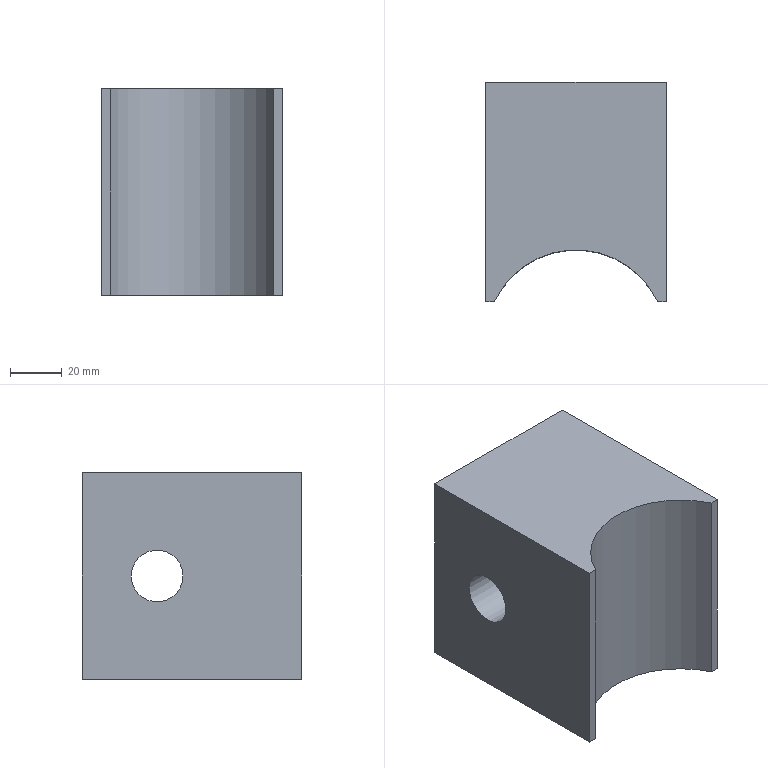Part | NX | features 护邦千斤顶滑块 2 | 1 solid | 9 faces | box 70 x 85 x 80 mm | volume 381423 mm3 | plane 7 | cylinder 2 | commonest cylinder face diameters 20 x1 70 x1
STEP:
#1=CARTESIAN_POINT('',(0.,-39.,40.));
#2=VERTEX_POINT('',#1);
#3=CARTESIAN_POINT('',(0.,-29.,40.));
#4=DIRECTION('',(-1.,0.,0.));
#5=DIRECTION('',(0.,-1.,0.));
#6=AXIS2_PLACEMENT_3D('',#3,#4,#5);
#7=CIRCLE('',#6,10.);
#8=EDGE_CURVE('',#2,#2,#7,.T.);
#9=ORIENTED_EDGE('',*,*,#8,.F.);
#10=EDGE_LOOP('',(#9));
#11=FACE_BOUND('',#10,.T.);
#12=CARTESIAN_POINT('',(0.,0.,0.));
#13=VERTEX_POINT('',#12);
#14=CARTESIAN_POINT('',(0.,-85.,0.));
#15=VERTEX_POINT('',#14);
#16=CARTESIAN_POINT('',(0.,0.,0.));
#17=DIRECTION('',(0.,-1.,0.));
#18=VECTOR('',#17,1000.);
#19=LINE('',#16,#18);
#20=EDGE_CURVE('',#13,#15,#19,.T.);
#21=ORIENTED_EDGE('',*,*,#20,.T.);
#22=CARTESIAN_POINT('',(0.,-85.,80.));
#23=VERTEX_POINT('',#22);
#24=CARTESIAN_POINT('',(0.,-85.,80.));
#25=DIRECTION('',(0.,0.,-1.));
#26=VECTOR('',#25,1000.);
#27=LINE('',#24,#26);
#28=EDGE_CURVE('',#23,#15,#27,.T.);
#29=ORIENTED_EDGE('',*,*,#28,.F.);
#30=CARTESIAN_POINT('',(0.,0.,80.));
#31=VERTEX_POINT('',#30);
#32=CARTESIAN_POINT('',(0.,0.,80.));
#33=DIRECTION('',(0.,-1.,0.));
#34=VECTOR('',#33,1000.);
#35=LINE('',#32,#34);
#36=EDGE_CURVE('',#31,#23,#35,.T.);
#37=ORIENTED_EDGE('',*,*,#36,.F.);
#38=CARTESIAN_POINT('',(0.,0.,80.));
#39=DIRECTION('',(0.,0.,-1.));
#40=VECTOR('',#39,1000.);
#41=LINE('',#38,#40);
#42=EDGE_CURVE('',#31,#13,#41,.T.);
#43=ORIENTED_EDGE('',*,*,#42,.T.);
#44=EDGE_LOOP('',(#21,#29,#37,#43));
#45=FACE_BOUND('',#44,.T.);
#46=CARTESIAN_POINT('',(0.,0.,80.));
#47=DIRECTION('',(1.,0.,0.));
#48=DIRECTION('',(0.,1.,0.));
#49=AXIS2_PLACEMENT_3D('',#46,#47,#48);
#50=PLANE('',#49);
#51=ADVANCED_FACE('',(#11,#45),#50,.F.);
#52=CARTESIAN_POINT('',(3.377,-85.,0.));
#53=VERTEX_POINT('',#52);
#54=CARTESIAN_POINT('',(0.,-85.,0.));
#55=DIRECTION('',(1.,0.,0.));
#56=VECTOR('',#55,1000.);
#57=LINE('',#54,#56);
#58=EDGE_CURVE('',#15,#53,#57,.T.);
#59=ORIENTED_EDGE('',*,*,#58,.T.);
#60=CARTESIAN_POINT('',(3.377,-85.,80.));
#61=VERTEX_POINT('',#60);
#62=CARTESIAN_POINT('',(3.377,-85.,80.));
#63=DIRECTION('',(0.,0.,-1.));
#64=VECTOR('',#63,1000.);
#65=LINE('',#62,#64);
#66=EDGE_CURVE('',#61,#53,#65,.T.);
#67=ORIENTED_EDGE('',*,*,#66,.F.);
#68=CARTESIAN_POINT('',(0.,-85.,80.));
#69=DIRECTION('',(1.,0.,0.));
#70=VECTOR('',#69,1000.);
#71=LINE('',#68,#70);
#72=EDGE_CURVE('',#23,#61,#71,.T.);
#73=ORIENTED_EDGE('',*,*,#72,.F.);
#74=ORIENTED_EDGE('',*,*,#28,.T.);
#75=EDGE_LOOP('',(#59,#67,#73,#74));
#76=FACE_BOUND('',#75,.T.);
#77=CARTESIAN_POINT('',(0.,-85.,80.));
#78=DIRECTION('',(0.,1.,0.));
#79=DIRECTION('',(0.,0.,1.));
#80=AXIS2_PLACEMENT_3D('',#77,#78,#79);
#81=PLANE('',#80);
#82=ADVANCED_FACE('',(#76),#81,.F.);
#83=CARTESIAN_POINT('',(66.623,-85.,0.));
#84=VERTEX_POINT('',#83);
#85=CARTESIAN_POINT('',(35.,-100.,0.));
#86=DIRECTION('',(0.,0.,-1.));
#87=DIRECTION('',(1.,0.,0.));
#88=AXIS2_PLACEMENT_3D('',#85,#86,#87);
#89=CIRCLE('',#88,35.);
#90=EDGE_CURVE('',#53,#84,#89,.T.);
#91=ORIENTED_EDGE('',*,*,#90,.T.);
#92=CARTESIAN_POINT('',(66.623,-85.,80.));
#93=VERTEX_POINT('',#92);
#94=CARTESIAN_POINT('',(66.623,-85.,80.));
#95=DIRECTION('',(0.,0.,-1.));
#96=VECTOR('',#95,1000.);
#97=LINE('',#94,#96);
#98=EDGE_CURVE('',#93,#84,#97,.T.);
#99=ORIENTED_EDGE('',*,*,#98,.F.);
#100=CARTESIAN_POINT('',(35.,-100.,80.));
#101=DIRECTION('',(0.,0.,-1.));
#102=DIRECTION('',(1.,0.,0.));
#103=AXIS2_PLACEMENT_3D('',#100,#101,#102);
#104=CIRCLE('',#103,35.);
#105=EDGE_CURVE('',#61,#93,#104,.T.);
#106=ORIENTED_EDGE('',*,*,#105,.F.);
#107=ORIENTED_EDGE('',*,*,#66,.T.);
#108=EDGE_LOOP('',(#91,#99,#106,#107));
#109=FACE_BOUND('',#108,.T.);
#110=CARTESIAN_POINT('',(35.,-100.,80.));
#111=DIRECTION('',(0.,0.,-1.));
#112=DIRECTION('',(-1.,0.,0.));
#113=AXIS2_PLACEMENT_3D('',#110,#111,#112);
#114=CYLINDRICAL_SURFACE('',#113,35.);
#115=ADVANCED_FACE('',(#109),#114,.F.);
#116=CARTESIAN_POINT('',(70.,-85.,0.));
#117=VERTEX_POINT('',#116);
#118=CARTESIAN_POINT('',(66.623,-85.,0.));
#119=DIRECTION('',(1.,0.,0.));
#120=VECTOR('',#119,1000.);
#121=LINE('',#118,#120);
#122=EDGE_CURVE('',#84,#117,#121,.T.);
#123=ORIENTED_EDGE('',*,*,#122,.T.);
#124=CARTESIAN_POINT('',(70.,-85.,80.));
#125=VERTEX_POINT('',#124);
#126=CARTESIAN_POINT('',(70.,-85.,80.));
#127=DIRECTION('',(0.,0.,-1.));
#128=VECTOR('',#127,1000.);
#129=LINE('',#126,#128);
#130=EDGE_CURVE('',#125,#117,#129,.T.);
#131=ORIENTED_EDGE('',*,*,#130,.F.);
#132=CARTESIAN_POINT('',(66.623,-85.,80.));
#133=DIRECTION('',(1.,0.,0.));
#134=VECTOR('',#133,1000.);
#135=LINE('',#132,#134);
#136=EDGE_CURVE('',#93,#125,#135,.T.);
#137=ORIENTED_EDGE('',*,*,#136,.F.);
#138=ORIENTED_EDGE('',*,*,#98,.T.);
#139=EDGE_LOOP('',(#123,#131,#137,#138));
#140=FACE_BOUND('',#139,.T.);
#141=CARTESIAN_POINT('',(66.623,-85.,80.));
#142=DIRECTION('',(0.,1.,0.));
#143=DIRECTION('',(0.,0.,1.));
#144=AXIS2_PLACEMENT_3D('',#141,#142,#143);
#145=PLANE('',#144);
#146=ADVANCED_FACE('',(#140),#145,.F.);
#147=CARTESIAN_POINT('',(70.,-39.,40.));
#148=VERTEX_POINT('',#147);
#149=CARTESIAN_POINT('',(70.,-29.,40.));
#150=DIRECTION('',(-1.,0.,0.));
#151=DIRECTION('',(0.,-1.,0.));
#152=AXIS2_PLACEMENT_3D('',#149,#150,#151);
#153=CIRCLE('',#152,10.);
#154=EDGE_CURVE('',#148,#148,#153,.T.);
#155=ORIENTED_EDGE('',*,*,#154,.T.);
#156=EDGE_LOOP('',(#155));
#157=FACE_BOUND('',#156,.T.);
#158=CARTESIAN_POINT('',(70.,0.,0.));
#159=VERTEX_POINT('',#158);
#160=CARTESIAN_POINT('',(70.,0.,0.));
#161=DIRECTION('',(0.,1.,0.));
#162=VECTOR('',#161,1000.);
#163=LINE('',#160,#162);
#164=EDGE_CURVE('',#117,#159,#163,.T.);
#165=ORIENTED_EDGE('',*,*,#164,.T.);
#166=CARTESIAN_POINT('',(70.,0.,80.));
#167=VERTEX_POINT('',#166);
#168=CARTESIAN_POINT('',(70.,0.,80.));
#169=DIRECTION('',(0.,0.,-1.));
#170=VECTOR('',#169,1000.);
#171=LINE('',#168,#170);
#172=EDGE_CURVE('',#167,#159,#171,.T.);
#173=ORIENTED_EDGE('',*,*,#172,.F.);
#174=CARTESIAN_POINT('',(70.,0.,80.));
#175=DIRECTION('',(0.,1.,0.));
#176=VECTOR('',#175,1000.);
#177=LINE('',#174,#176);
#178=EDGE_CURVE('',#125,#167,#177,.T.);
#179=ORIENTED_EDGE('',*,*,#178,.F.);
#180=ORIENTED_EDGE('',*,*,#130,.T.);
#181=EDGE_LOOP('',(#165,#173,#179,#180));
#182=FACE_BOUND('',#181,.T.);
#183=CARTESIAN_POINT('',(70.,0.,80.));
#184=DIRECTION('',(-1.,0.,0.));
#185=DIRECTION('',(0.,-1.,0.));
#186=AXIS2_PLACEMENT_3D('',#183,#184,#185);
#187=PLANE('',#186);
#188=ADVANCED_FACE('',(#157,#182),#187,.F.);
#189=CARTESIAN_POINT('',(0.,0.,0.));
#190=DIRECTION('',(-1.,0.,0.));
#191=VECTOR('',#190,1000.);
#192=LINE('',#189,#191);
#193=EDGE_CURVE('',#159,#13,#192,.T.);
#194=ORIENTED_EDGE('',*,*,#193,.T.);
#195=ORIENTED_EDGE('',*,*,#42,.F.);
#196=CARTESIAN_POINT('',(0.,0.,80.));
#197=DIRECTION('',(-1.,0.,0.));
#198=VECTOR('',#197,1000.);
#199=LINE('',#196,#198);
#200=EDGE_CURVE('',#167,#31,#199,.T.);
#201=ORIENTED_EDGE('',*,*,#200,.F.);
#202=ORIENTED_EDGE('',*,*,#172,.T.);
#203=EDGE_LOOP('',(#194,#195,#201,#202));
#204=FACE_BOUND('',#203,.T.);
#205=CARTESIAN_POINT('',(0.,0.,80.));
#206=DIRECTION('',(0.,-1.,0.));
#207=DIRECTION('',(0.,0.,-1.));
#208=AXIS2_PLACEMENT_3D('',#205,#206,#207);
#209=PLANE('',#208);
#210=ADVANCED_FACE('',(#204),#209,.F.);
#211=ORIENTED_EDGE('',*,*,#36,.T.);
#212=ORIENTED_EDGE('',*,*,#72,.T.);
#213=ORIENTED_EDGE('',*,*,#105,.T.);
#214=ORIENTED_EDGE('',*,*,#136,.T.);
#215=ORIENTED_EDGE('',*,*,#178,.T.);
#216=ORIENTED_EDGE('',*,*,#200,.T.);
#217=EDGE_LOOP('',(#211,#212,#213,#214,#215,#216));
#218=FACE_BOUND('',#217,.T.);
#219=CARTESIAN_POINT('',(35.,-100.,80.));
#220=DIRECTION('',(0.,0.,1.));
#221=DIRECTION('',(1.,0.,0.));
#222=AXIS2_PLACEMENT_3D('',#219,#220,#221);
#223=PLANE('',#222);
#224=ADVANCED_FACE('',(#218),#223,.T.);
#225=ORIENTED_EDGE('',*,*,#20,.F.);
#226=ORIENTED_EDGE('',*,*,#193,.F.);
#227=ORIENTED_EDGE('',*,*,#164,.F.);
#228=ORIENTED_EDGE('',*,*,#122,.F.);
#229=ORIENTED_EDGE('',*,*,#90,.F.);
#230=ORIENTED_EDGE('',*,*,#58,.F.);
#231=EDGE_LOOP('',(#225,#226,#227,#228,#229,#230));
#232=FACE_BOUND('',#231,.T.);
#233=CARTESIAN_POINT('',(35.,-100.,0.));
#234=DIRECTION('',(0.,0.,1.));
#235=DIRECTION('',(1.,0.,0.));
#236=AXIS2_PLACEMENT_3D('',#233,#234,#235);
#237=PLANE('',#236);
#238=ADVANCED_FACE('',(#232),#237,.F.);
#239=ORIENTED_EDGE('',*,*,#8,.T.);
#240=EDGE_LOOP('',(#239));
#241=FACE_BOUND('',#240,.T.);
#242=ORIENTED_EDGE('',*,*,#154,.F.);
#243=EDGE_LOOP('',(#242));
#244=FACE_BOUND('',#243,.T.);
#245=CARTESIAN_POINT('',(80.,-29.,40.));
#246=DIRECTION('',(-1.,0.,0.));
#247=DIRECTION('',(0.,-1.,0.));
#248=AXIS2_PLACEMENT_3D('',#245,#246,#247);
#249=CYLINDRICAL_SURFACE('',#248,10.);
#250=ADVANCED_FACE('',(#241,#244),#249,.F.);
#251=CLOSED_SHELL('',(#51,#82,#115,#146,#188,#210,#224,#238,#250));
#252=MANIFOLD_SOLID_BREP('',#251);
#253=(LENGTH_UNIT()NAMED_UNIT(*)SI_UNIT(.MILLI.,.METRE.));
#254=UNCERTAINTY_MEASURE_WITH_UNIT(LENGTH_MEASURE(0.00001),#253,'','');
#255=(NAMED_UNIT(*)PLANE_ANGLE_UNIT()SI_UNIT($,.RADIAN.));
#256=(NAMED_UNIT(*)SI_UNIT($,.STERADIAN.)SOLID_ANGLE_UNIT());
#257=(GEOMETRIC_REPRESENTATION_CONTEXT(3)GLOBAL_UNCERTAINTY_ASSIGNED_CONTEXT((#254))GLOBAL_UNIT_ASSIGNED_CONTEXT((#253,#255,#256))REPRESENTATION_CONTEXT('',''));
#258=ADVANCED_BREP_SHAPE_REPRESENTATION('',(#252),#257);